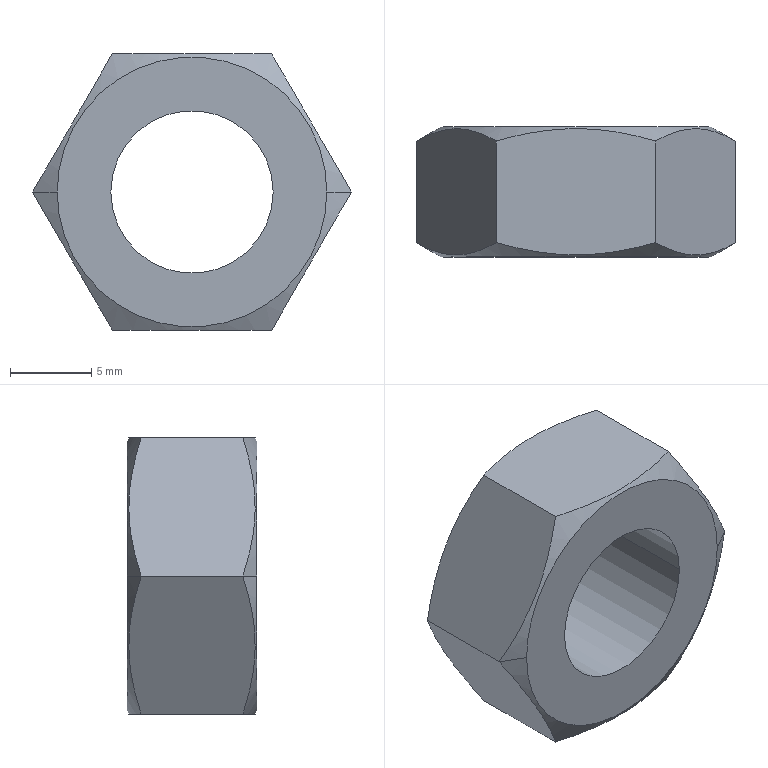Part | STEP file | LIB_27044239_HEX_NUT_M10_SIMPLE | 1 solid | 14 faces | box 19.63 x 8 x 17 mm | volume 1357 mm3 | plane 8 | cone 4 | cylinder 2 | commonest cylinder face diameters 10 x2